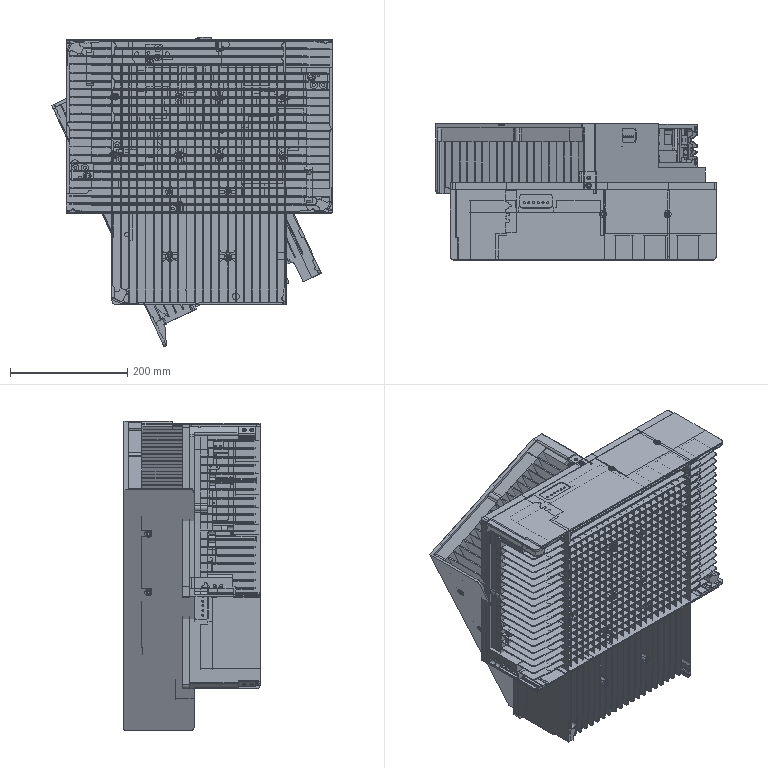CAM job | NX | 3-axis milling, drilling | stock box 478.438 x 232 x 527.231 mm
Tools:
number,name,description,diameter,corner_radius,flute_length,length,flutes
1,D10_J,Milling Tool-5 Parameters,10.0,0.0,50.0,50.0,2
2,CR_8,Countersink,8.0,0.0,0.0,60.0,2
3,CR_4,Countersink,4.0,0.0,0.0,60.0,2
4,D6_J,Milling Tool-5 Parameters,6.0,0.0,50.0,50.0,2
5,D4_J,Milling Tool-5 Parameters,4.0,0.0,50.0,60.0,2
6,Z2.6,Drilling Tool,2.6,0.0,30.0,50.0,2
7,M3,Drilling Tool,3.0,0.0,30.0,50.0,2
8,Z5.2,Drilling Tool,5.2,0.0,50.0,70.0,2
9,M6,Drilling Tool,6.0,0.0,30.0,50.0,2
17,M12X1.5,Drilling Tool,12.0,0.0,30.0,50.0,2
16,GSLT-M5,Drilling Tool,6.0,0.0,30.0,50.0,2
10,CR_3,Milling Tool-5 Parameters,0.3,0.0,50.0,75.0,2
11,Z10.5,Drilling Tool,10.5,0.0,50.0,70.0,2
12,D2.5_J,Milling Tool-5 Parameters,2.5,0.0,50.0,50.0,2
14,Z3.8,Drilling Tool,3.8,0.0,35.0,50.0,2
15,D3_J,Milling Tool-5 Parameters,3.0,0.0,30.0,50.0,2
16,D8R1,Milling Tool-5 Parameters,8.0,1.0,50.0,75.0,2
Operations:
program,operation,operation_type,tool,method,geometry_group,spindle_rpm,surface_speed,feed_per_tooth,feed_cut,feed_plunge,cut_length_mm,path_length_mm,cut_time_min,machine_time_min
W27,PLANAR_PROFILE_COPY_COPY_3_COPY_COPY,PlanarMilling,D10_J,METHOD,G54,7500.0,0.0,0.1,1500.0,100.0,47.6,102.4,0.0317,0.0372
W27,PLANAR_PROFILE_COPY_COPY_3_COPY,PlanarMilling,D10_J,METHOD,G54,7500.0,0.0,0.1,1500.0,100.0,186.0,896.277,0.124,0.195
W27,PX_1_COPY,SurfaceContour,D10_J,METHOD,G54,7500.0,69.0,0.2727,2500.0,100.0,630.219,773.27,0.2521,0.2664
W27,PLANAR_PROFILE_COPY,PlanarMilling,D10_J,METHOD,G54,7500.0,0.0,0.1667,2500.0,100.0,2403.044,2529.843,0.9612,0.9739
W27,PLANAR_PROFILE_COPY_COPY_2,PlanarMilling,D10_J,METHOD,G54,7500.0,0.0,0.1667,2500.0,100.0,854.585,981.385,0.3418,0.3545
W27,PLANAR_PROFILE_COPY_COPY_2_COPY_1,PlanarMilling,D10_J,METHOD,G54,7500.0,0.0,0.1,1500.0,100.0,521.673,638.673,0.3478,0.3595
W27,PLANAR_PROFILE_COPY_COPY_2_COPY_1_COPY,PlanarMilling,D10_J,METHOD,G54,7500.0,0.0,0.1,1500.0,100.0,35.267,305.732,0.0235,0.0506
W27,PLANAR_PROFILE_COPY_COPY_2_COPY,PlanarMilling,D10_J,METHOD,G54,7500.0,0.0,0.1667,2500.0,100.0,943.144,1069.944,0.3773,0.3899
W27,PLANAR_PROFILE_COPY_COPY_2_COPY_COPY,PlanarMilling,D10_J,METHOD,G54,7500.0,0.0,0.1667,2500.0,100.0,345.704,454.504,0.1383,0.1492
W27,PLANAR_PROFILE_COPY_COPY_3_COPY_2,PlanarMilling,D10_J,METHOD,G54,7500.0,0.0,0.1,1500.0,100.0,118.82,243.82,0.0792,0.0917
W27,PLANAR_PROFILE_COPY_COPY_3,PlanarMilling,D10_J,METHOD,G54,7500.0,0.0,0.1,1500.0,100.0,122.525,247.525,0.0817,0.0942
W27,PLANAR_MILL_COPY_COPY_COPY_1_COPY_COPY_COPY_1_COPY_COPY_COPY_COPY_1,PlanarMilling,D10_J,METHOD,G54,8000.0,0.0,0.2333,1500.0,100.0,736.062,861.062,0.4907,0.5032
W27,FACE_MILLING_COPY_COPY_COPY_1_COPY_3,FaceMilling,D10_J,METHOD,G54,8000.0,0.0,0.2333,1500.0,100.0,392.088,614.324,0.2614,0.2836
W27,FACE_MILLING_COPY_COPY_COPY_1_COPY_3_COPY,FaceMilling,D10_J,METHOD,G54,8000.0,0.0,0.2333,1500.0,100.0,317.508,966.305,0.2117,0.2766
W27,PX_1_COPY_COPY_1,SurfaceContour,D10_J,METHOD,G54,7500.0,69.0,0.2727,2500.0,100.0,485.34,561.34,0.1941,0.2017
W27,PLANAR_MILL_COPY_COPY_COPY_1_COPY_COPY_COPY_1_COPY_COPY_COPY_COPY_1_COPY,PlanarMilling,D10_J,METHOD,G54,8000.0,0.0,0.2333,1500.0,100.0,791.735,911.235,0.5278,0.5398
W27,PLANAR_PROFILE_COPY_COPY_COPY_COPY_COPY_COPY_COPY_1,PlanarMilling,D10_J,METHOD,G54,7500.0,0.0,0.08,1200.0,100.0,19.0,122.0,0.0158,0.0261
W27,DG_1_COPY_COPY_2_COPY,ZLevelMilling,D10_J,METHOD,G54,8500.0,0.0,0.1471,2500.0,100.0,935.965,1017.165,0.3744,0.3825
W27,FACE_MILLING_COPY_COPY_COPY_1_COPY_3_COPY_COPY,FaceMilling,D10_J,METHOD,G54,8000.0,0.0,0.2333,1500.0,100.0,196.507,801.996,0.131,0.1916
W27,DG_1_COPY_COPY_2_COPY_COPY_COPY_1,ZLevelMilling,D10_J,METHOD,G54,8500.0,0.0,0.1471,2500.0,100.0,955.229,1070.629,0.3821,0.3936
W27,DG_1_COPY_COPY_2_COPY_COPY,ZLevelMilling,D10_J,METHOD,G54,8500.0,0.0,0.1471,2500.0,100.0,1318.762,1434.162,0.5275,0.539
W27,HOLE_MILLING_3,CylinderMilling,D10_J,METHOD,G54,8000.0,0.0,0.0,2500.0,100.0,930.302,990.802,0.3721,0.3782
W27,HOLE_MILLING_3_COPY,CylinderMilling,D10_J,METHOD,G54,8000.0,0.0,0.0,1200.0,100.0,21.677,103.677,0.0181,0.0263
W27_COPY,HOLE_MILLING_3_COPY_1,CylinderMilling,D4_J,METHOD,G54,8000.0,0.0,0.0,2500.0,100.0,1240.867,1371.367,0.4963,0.5094
W27_COPY,HOLE_MILLING_3_COPY_1_COPY,CylinderMilling,D4_J,METHOD,G54,8000.0,0.0,0.0,2500.0,100.0,906.876,1037.376,0.3628,0.3758
W27_COPY,PLANAR_PROFILE_COPY_COPY_3_COPY_1,PlanarMilling,D4_J,METHOD,G54,7500.0,0.0,0.1,1500.0,100.0,511.204,656.514,0.3408,0.3553
W27_COPY,PLANAR_PROFILE_COPY_COPY_3_COPY_1_COPY,PlanarMilling,D4_J,METHOD,G54,7500.0,0.0,0.1,1500.0,100.0,176.817,227.742,0.1179,0.123
W65,ZK_1_COPY_COPY_4,Operation,CR_8,METHOD,G54,7500.0,0.0,0.0008,500.0,0.0,18.0,462.606,0.036,0.0805
W66,ZK_1_COPY_COPY_4_COPY,Operation,Z10.5,METHOD,G54,2000.0,0.0,0.0008,500.0,0.0,17.0,159.4,0.034,0.0482
W67,ZK_1_COPY_COPY_4_COPY_COPY,Operation,Z2.6,METHOD,G54,2000.0,0.0,0.0008,220.0,0.0,60.0,335.681,0.2727,0.3003
W68,DG_1_COPY_COPY_2_COPY_COPY_3,ZLevelMilling,D6_J,METHOD,G54,8500.0,0.0,0.0882,1500.0,100.0,967.287,1048.487,0.6449,0.653
W68,DG_1_COPY_COPY_2_COPY_COPY_COPY,ZLevelMilling,D6_J,METHOD,G54,8500.0,0.0,0.0882,1500.0,100.0,1853.936,1969.336,1.236,1.248
W68,DG_1_COPY_COPY_2_COPY_COPY_COPY_COPY,ZLevelMilling,D6_J,METHOD,G54,8500.0,0.0,0.1471,2500.0,100.0,663.86,1057.072,0.2655,0.3049
W68,DG_1_COPY_COPY_2_COPY_COPY_COPY_COPY_COPY,ZLevelMilling,D6_J,METHOD,G54,8500.0,0.0,0.1176,2000.0,100.0,1683.898,1802.898,0.8419,0.8538
W68,PLANAR_PROFILE_COPY_COPY_COPY_COPY_COPY_COPY,PlanarMilling,D6_J,METHOD,G54,7500.0,0.0,0.08,1200.0,100.0,118.212,275.212,0.0985,0.1142
W68,DG_1_COPY_COPY_2_COPY_COPY_COPY_COPY_COPY_COPY_COPY_COPY_COPY,ZLevelMilling,D6_J,METHOD,G54,8500.0,0.0,0.0882,1500.0,100.0,270.01,375.01,0.18,0.1905
W68,DG_1_COPY_COPY_2_COPY_COPY_COPY_COPY_COPY_COPY,ZLevelMilling,D6_J,METHOD,G54,8500.0,0.0,0.0882,1500.0,100.0,1167.785,1564.689,0.7785,0.8182
W68,DG_1_COPY_COPY_2_COPY_COPY_COPY_COPY_COPY_COPY_COPY,ZLevelMilling,D6_J,METHOD,G54,8500.0,0.0,0.0882,1500.0,100.0,434.204,683.626,0.2895,0.3144
W68,DG_1_COPY_COPY_2_COPY_COPY_COPY_COPY_COPY_COPY_COPY_COPY,ZLevelMilling,D6_J,METHOD,G54,8500.0,0.0,0.0882,1500.0,100.0,215.619,326.369,0.1437,0.1548
W68,PLANAR_PROFILE_COPY_COPY_COPY_COPY_COPY_COPY_COPY,PlanarMilling,D6_J,METHOD,G54,7500.0,0.0,0.1667,2500.0,100.0,355.477,496.477,0.1422,0.1563
W68,PLANAR_PROFILE_COPY_COPY_COPY_COPY_COPY_COPY_COPY_COPY,PlanarMilling,D6_J,METHOD,G54,7500.0,0.0,0.1667,2500.0,100.0,530.789,671.789,0.2123,0.2264
W68,PLANAR_MILL_COPY_COPY_COPY_1_COPY_COPY_COPY_1_COPY_COPY_COPY_COPY_1_COPY_1,PlanarMilling,D6_J,METHOD,G54,8000.0,0.0,0.2333,1500.0,100.0,525.616,934.317,0.3504,0.3913
W69,ZK_1_COPY_COPY_4_COPY_COPY_COPY,Operation,CR_8,METHOD,G54,7500.0,0.0,0.0008,500.0,0.0,17.5,250.681,0.035,0.0583
W71,ZK_1_COPY_COPY_4_COPY_COPY_COPY_1,Operation,M3,METHOD,G54,2000.0,0.0,0.0001,0.5,0.0,47.5,310.681,95.0,95.026
W72,DJ_COPY_COPY,PlanarMilling,CR_4,METHOD,G54,8500.0,0.0,0.1471,2500.0,100.0,130.576,348.576,0.0522,0.074
W72,DJ_COPY_COPY_COPY_1,PlanarMilling,CR_4,METHOD,G54,8500.0,0.0,0.1471,2500.0,100.0,82.266,136.266,0.0329,0.0383
W72,DJ_COPY_COPY_COPY,PlanarMilling,CR_4,METHOD,G54,8500.0,0.0,0.1471,2500.0,100.0,97.623,360.364,0.039,0.0653
W72,DJ_COPY_COPY_COPY_COPY,PlanarMilling,CR_4,METHOD,G54,8500.0,0.0,0.1471,2500.0,100.0,53.559,159.959,0.0214,0.0321
W72,DJ_COPY_COPY_COPY_COPY_COPY_COPY,PlanarMilling,CR_4,METHOD,G54,8500.0,0.0,0.1471,2500.0,100.0,18.398,120.798,0.0074,0.0176
W72,DJ_COPY_COPY_COPY_COPY_COPY,PlanarMilling,CR_4,METHOD,G54,8500.0,0.0,0.1471,2500.0,100.0,168.49,275.19,0.0674,0.0781
W74,DJ_COPY_COPY_COPY_2,PlanarMilling,CR_3,METHOD,G54,8500.0,0.0,0.0588,1000.0,100.0,316.906,2018.803,0.3169,0.4871
W74,DJ_COPY_COPY_COPY_2_COPY,PlanarMilling,CR_3,METHOD,G54,8500.0,0.0,0.0588,1000.0,100.0,72.086,843.529,0.0721,0.1492
W74,DJ_COPY_COPY_COPY_2_COPY_2,PlanarMilling,CR_3,METHOD,G54,8500.0,0.0,0.0588,1000.0,100.0,14.005,128.805,0.014,0.0255
W73,ZK_1_COPY_COPY_4_COPY_COPY_1,Operation,M12X1.5,METHOD,G54,2000.0,0.0,0.0004,1.5,0.0,12.0,149.4,8.0,8.014
W73_COPY,PLANAR_PROFILE_COPY_COPY_3_COPY_1_COPY_COPY,PlanarMilling,D4_J,METHOD,G54,7500.0,0.0,0.1,1500.0,100.0,176.817,227.742,0.1179,0.123
W73_COPY,DJ_COPY_COPY_COPY_2_COPY_2_COPY,PlanarMilling,CR_3,METHOD,G54,8500.0,0.0,0.0588,1000.0,100.0,14.005,128.805,0.014,0.0255
W73_COPY,DG_1_COPY_COPY_2_COPY_COPY_COPY_COPY_COPY_1,ZLevelMilling,D8R1,METHOD,G54,8000.0,251.0,0.125,2000.0,100.0,469.925,596.616,0.235,0.2476
W02,FACE_MILLING_COPY_COPY_COPY_1_COPY_3_COPY_1,FaceMilling,D10_J,METHOD,G54,8000.0,0.0,0.2333,1500.0,100.0,116.203,294.447,0.0775,0.0953
W02,PLANAR_PROFILE_COPY_COPY_3_COPY_COPY_COPY,PlanarMilling,D10_J,METHOD,G54,8000.0,0.0,0.1562,2500.0,100.0,302.884,502.873,0.1212,0.1412
W02,PLANAR_MILL_COPY_COPY_COPY_1_COPY_COPY_COPY_1_COPY_COPY_COPY_COPY_1_COPY_2,PlanarMilling,D10_J,METHOD,G54,8000.0,0.0,0.2333,1500.0,100.0,652.682,814.615,0.4351,0.4513
W03,HOLE_MILLING,CylinderMilling,D4_J,METHOD,G54,8000.0,100.0,0.0938,1500.0,100.0,194.81,385.41,0.1299,0.1489
W04,ZK_1_COPY_COPY_4_COPY_1,Operation,CR_8,METHOD,G54,7500.0,0.0,0.0008,500.0,0.0,6.0,166.618,0.012,0.0281
W05,ZK_1_COPY_COPY_4_COPY_1_COPY,Operation,Z5.2,METHOD,G54,3000.0,0.0,0.0008,300.0,0.0,32.0,218.618,0.1067,0.1253
W06,ZK_1_COPY_COPY_4_COPY_1_COPY_1,Operation,CR_8,METHOD,G54,7500.0,0.0,0.0008,500.0,0.0,10.0,174.618,0.02,0.0365
W12,ZK_1_COPY_COPY_4_COPY_1_COPY_COPY,Operation,M6,METHOD,G54,2000.0,0.0,0.0008,1.0,0.0,26.0,206.618,26.0,26.018
W13,DJ_COPY_COPY_COPY_3,PlanarMilling,CR_4,METHOD,G54,8500.0,0.0,0.1471,2500.0,100.0,140.407,407.063,0.0562,0.0828
W01,PLANAR_MILL_COPY_COPY_COPY_1_COPY_COPY_COPY_1_COPY_COPY_COPY_COPY_1_COPY_COPY,PlanarMilling,D10_J,METHOD,G54,8000.0,0.0,0.2333,1500.0,100.0,1618.01,1674.01,1.079,1.084
W01,PLANAR_MILL_COPY_COPY_COPY_1_COPY_COPY_COPY_1_COPY_COPY_COPY_COPY_1_COPY_COPY_COPY,PlanarMilling,D10_J,METHOD,G54,8000.0,0.0,0.2333,1500.0,100.0,1170.544,1221.544,0.7804,0.7855
W01,PLANAR_MILL_COPY_COPY_COPY_1_COPY_COPY_COPY_1_COPY_COPY_COPY_COPY_1_COPY_COPY_COPY_COPY,PlanarMilling,D10_J,METHOD,G54,8000.0,0.0,0.2333,1500.0,100.0,1163.605,1226.105,0.7757,0.782
W01,FACE_MILLING_COPY_COPY_COPY_1_COPY_3_COPY_2,FaceMilling,D10_J,METHOD,G54,8000.0,0.0,0.2333,1500.0,100.0,1782.698,2104.083,1.188,1.221
W01,CAVITY_MILL,CavityMilling,D10_J,METHOD,G54,7500.0,235.0,0.2333,3500.0,100.0,47087.83,49581.844,13.454,13.703
W01,FACE_MILLING_COPY_COPY_COPY_1_COPY_3_COPY_2_COPY,FaceMilling,D10_J,METHOD,G54,8000.0,0.0,0.2333,1500.0,100.0,1344.186,2793.189,0.8961,1.041
W07,HOLE_MILLING_1,CylinderMilling,D6_J,METHOD,G54,8000.0,0.0,0.0,1500.0,100.0,216.836,303.836,0.1446,0.1533
W07,CAVITY_MILL_COPY,CavityMilling,D6_J,METHOD,G54,8000.0,150.0,0.1875,3000.0,100.0,16037.881,26925.285,5.346,6.435
W07,FACE_MILLING_COPY_COPY_COPY_1_COPY_3_COPY_2_COPY_COPY,FaceMilling,D6_J,METHOD,G54,8000.0,0.0,0.2333,1500.0,100.0,858.792,2126.935,0.5725,0.6993
W07,PLANAR_PROFILE_COPY_COPY_3_COPY_COPY_1_COPY_3,PlanarMilling,D6_J,METHOD,G54,7500.0,0.0,0.1,1500.0,100.0,88.083,162.083,0.0587,0.0661
W07,FACE_MILLING_COPY_COPY_COPY_1_COPY_3_COPY_2_COPY_COPY_COPY,FaceMilling,D6_J,METHOD,G54,8000.0,0.0,0.2333,1500.0,100.0,608.245,1917.272,0.4055,0.5364
W07,PLANAR_PROFILE_COPY_COPY_3_COPY_COPY_1,PlanarMilling,D6_J,METHOD,G54,7500.0,0.0,0.1,1500.0,100.0,568.85,773.65,0.3792,0.3997
W07,PLANAR_PROFILE_COPY_COPY_3_COPY_COPY_1_COPY,PlanarMilling,D6_J,METHOD,G54,7500.0,0.0,0.1,1500.0,100.0,21.283,137.683,0.0142,0.0258
W07,PLANAR_PROFILE_COPY_COPY_3_COPY_COPY_1_COPY_1,PlanarMilling,D6_J,METHOD,G54,7500.0,0.0,0.1,1500.0,100.0,402.733,998.933,0.2685,0.3281
W07,FACE_MILLING_COPY_COPY_COPY_1_COPY_3_COPY_2_COPY_COPY_COPY_3,FaceMilling,D6_J,METHOD,G54,8000.0,0.0,0.2188,3500.0,100.0,1632.647,1869.109,0.4665,0.4901
W07,FACE_MILLING_COPY_COPY_COPY_1_COPY_3_COPY_2_COPY_COPY_COPY_3_COPY,FaceMilling,D6_J,METHOD,G54,8000.0,0.0,0.2333,1500.0,100.0,356.654,394.454,0.2378,0.2415
W07,DG_1_COPY_COPY_2_COPY_COPY_1,ZLevelMilling,D6_J,METHOD,G54,8500.0,0.0,0.1471,2500.0,100.0,2918.479,5757.108,1.167,1.451
W07,PX_1_COPY_COPY,SurfaceContour,D6_J,METHOD,G54,7500.0,69.0,0.2727,2500.0,100.0,3224.559,3765.461,1.29,1.344
W08,FACE_MILLING_COPY_COPY_COPY_1_COPY_3_COPY_2_COPY_COPY_COPY_2_COPY_COPY,FaceMilling,D4_J,METHOD,G54,8000.0,0.0,0.2333,1500.0,100.0,125.867,468.46,0.0839,0.1182
W08,DG_1_COPY_COPY_2_COPY_COPY_1_COPY,ZLevelMilling,D4_J,METHOD,G54,8500.0,0.0,0.1471,2500.0,100.0,6784.364,7077.339,2.714,2.743
W08,DG_1_COPY_COPY_2_COPY_COPY_1_COPY_COPY,ZLevelMilling,D4_J,METHOD,G54,8500.0,0.0,0.1471,2500.0,100.0,1548.077,1712.238,0.6192,0.6356
W08,PLANAR_PROFILE_COPY_COPY_3_COPY_COPY_1_COPY_2,PlanarMilling,D4_J,METHOD,G54,7500.0,0.0,0.1,1500.0,100.0,522.0,627.444,0.348,0.3585
W08,PLANAR_PROFILE_COPY_COPY_3_COPY_COPY_1_COPY_2_COPY,PlanarMilling,D4_J,METHOD,G54,7500.0,0.0,0.1667,2500.0,100.0,2057.213,2378.148,0.8229,0.855
W08,FACE_MILLING_COPY_COPY_COPY_1_COPY_3_COPY_2_COPY_COPY_COPY_1,FaceMilling,D4_J,METHOD,G54,8000.0,0.0,0.2333,1500.0,100.0,99.01,362.088,0.066,0.0923
W08,PLANAR_PROFILE_COPY_COPY_3_COPY_COPY_1_COPY_2_COPY_COPY,PlanarMilling,D4_J,METHOD,G54,7500.0,0.0,0.1,1500.0,100.0,43.783,133.783,0.0292,0.0382
W08,PLANAR_PROFILE_COPY_COPY_3_COPY_COPY_1_COPY_3_COPY,PlanarMilling,D4_J,METHOD,G54,7500.0,0.0,0.1,1500.0,100.0,95.954,169.954,0.064,0.0714
W08,PX_1_COPY_COPY_COPY,SurfaceContour,D4_J,METHOD,G54,7500.0,69.0,0.2727,2500.0,100.0,996.115,1109.056,0.3984,0.4097
W08,PX_1_COPY_COPY_COPY_COPY,SurfaceContour,D4_J,METHOD,G54,7500.0,69.0,0.1,1500.0,100.0,92.736,199.936,0.0618,0.0725
W08,PLANAR_PROFILE_COPY_COPY_3_COPY_COPY_1_COPY_3_COPY_1,PlanarMilling,D4_J,METHOD,G54,7500.0,0.0,0.1,1500.0,100.0,28.283,72.283,0.0189,0.0233
W14,PLANAR_MILL_COPY_COPY_COPY_1_COPY_COPY_COPY_1_COPY_COPY_COPY_COPY_1_COPY_COPY_COPY_COPY_COPY_COPY_COPY_1_COPY_COPY,PlanarMilling,D2.5_J,METHOD,G54,8000.0,0.0,0.0938,1500.0,100.0,115.791,219.312,0.0772,0.0875
W14,PLANAR_MILL_COPY_COPY_COPY_1_COPY_COPY_COPY_1_COPY_COPY_COPY_COPY_1_COPY_COPY_COPY_COPY_COPY,PlanarMilling,D2.5_J,METHOD,G54,8000.0,0.0,0.1562,2500.0,100.0,5609.504,5689.004,2.244,2.252
W14,PLANAR_MILL_COPY_COPY_COPY_1_COPY_COPY_COPY_1_COPY_COPY_COPY_COPY_1_COPY_COPY_COPY_COPY_COPY_COPY,PlanarMilling,D2.5_J,METHOD,G54,8000.0,0.0,0.1562,2500.0,100.0,301.593,405.305,0.1206,0.131
W14,PLANAR_MILL_COPY_COPY_COPY_1_COPY_COPY_COPY_1_COPY_COPY_COPY_COPY_1_COPY_COPY_COPY_COPY_COPY_COPY_COPY,PlanarMilling,D2.5_J,METHOD,G54,8000.0,0.0,0.1562,2500.0,100.0,301.593,405.305,0.1206,0.131
W14,PLANAR_MILL_COPY_COPY_COPY_1_COPY_COPY_COPY_1_COPY_COPY_COPY_COPY_1_COPY_COPY_COPY_COPY_COPY_COPY_COPY_1,PlanarMilling,D2.5_J,METHOD,G54,8000.0,0.0,0.1562,2500.0,100.0,301.593,405.305,0.1206,0.131
W14,PLANAR_MILL_COPY_COPY_COPY_1_COPY_COPY_COPY_1_COPY_COPY_COPY_COPY_1_COPY_COPY_COPY_COPY_COPY_COPY_COPY_1_COPY,PlanarMilling,D2.5_J,METHOD,G54,8000.0,0.0,0.1562,2500.0,100.0,301.593,405.305,0.1206,0.131
W15,ZK_1_COPY_COPY_4_COPY_2,Operation,CR_8,METHOD,G54,7500.0,0.0,0.0008,500.0,0.0,42.0,602.9,0.084,0.1401
W16,ZK_1_COPY_COPY_4_COPY_COPY_COPY_2,Operation,Z2.6,METHOD,G54,2000.0,0.0,0.0008,220.0,0.0,24.0,190.859,0.1091,0.1258
W16,ZK_1_COPY_COPY_4_COPY_COPY_COPY_2_COPY,Operation,Z2.6,METHOD,G54,2000.0,0.0,0.0008,220.0,0.0,42.0,218.404,0.1909,0.2085
W25,ZK_1_COPY_COPY_4_COPY_COPY_COPY_2_COPY_COPY,Operation,Z3.8,METHOD,G54,2000.0,0.0,0.0008,220.0,0.0,30.0,192.034,0.1364,0.1526
W25,ZK_1_COPY_COPY_4_COPY_COPY_COPY_2_COPY_COPY_1,Operation,Z3.8,METHOD,G54,2000.0,0.0,0.0008,220.0,0.0,72.0,254.668,0.3273,0.3455
W26,HOLE_MILLING_2,CylinderMilling,D3_J,METHOD,G54,8000.0,0.0,0.0,1500.0,100.0,732.813,960.313,0.4885,0.5113
W26,DG_1_COPY_COPY_2_COPY_COPY_1_COPY_COPY_1,ZLevelMilling,D3_J,METHOD,G54,8500.0,0.0,0.1176,2000.0,100.0,538.012,737.175,0.269,0.2889
W28,ZK_1_COPY_COPY_4_COPY_COPY_COPY_2_COPY_COPY_2,Operation,CR_8,METHOD,G54,2000.0,0.0,0.0008,220.0,0.0,21.0,296.974,0.0955,0.1231
W28,ZK_1_COPY_COPY_4_COPY_COPY_COPY_2_COPY_COPY_COPY,Operation,CR_8,METHOD,G54,2000.0,0.0,0.0008,220.0,0.0,9.0,150.034,0.0409,0.055
W28,ZK_1_COPY_COPY_4_COPY_COPY_COPY_2_COPY_COPY_1_COPY,Operation,CR_8,METHOD,G54,2000.0,0.0,0.0008,220.0,0.0,23.4,157.468,0.1064,0.1198
W29,DJ_COPY_COPY_COPY_4,PlanarMilling,CR_4,METHOD,G54,8500.0,0.0,0.1471,2500.0,100.0,415.091,607.277,0.166,0.1853
W29,DJ_COPY_COPY_COPY_4_COPY,PlanarMilling,CR_4,METHOD,G54,8500.0,0.0,0.1471,2500.0,100.0,125.111,193.511,0.05,0.0569
W29,DJ_COPY_COPY_COPY_4_COPY_COPY,PlanarMilling,CR_4,METHOD,G54,8500.0,0.0,0.1471,2500.0,100.0,400.018,468.418,0.16,0.1668
W29,DJ_COPY_COPY_COPY_4_COPY_COPY_COPY,PlanarMilling,CR_4,METHOD,G54,8500.0,0.0,0.1471,2500.0,100.0,113.1,211.3,0.0452,0.0551
W29,DJ_COPY_COPY_COPY_4_COPY_COPY_COPY_COPY,PlanarMilling,CR_4,METHOD,G54,8500.0,0.0,0.1471,2500.0,100.0,65.996,146.797,0.0264,0.0345
W29,DJ_COPY_COPY_COPY_4_COPY_COPY_COPY_COPY_COPY,PlanarMilling,CR_4,METHOD,G54,8500.0,0.0,0.1471,2500.0,100.0,53.741,140.741,0.0215,0.0302
W29,DJ_COPY_COPY_COPY_4_COPY_COPY_COPY_COPY_COPY_COPY,PlanarMilling,CR_4,METHOD,G54,8500.0,0.0,0.1471,2500.0,100.0,113.785,358.999,0.0455,0.07
W30,DJ_COPY_COPY_COPY_2_COPY_1,PlanarMilling,CR_3,METHOD,G54,8500.0,0.0,0.0588,1000.0,100.0,110.225,766.258,0.1102,0.1758
W30,DJ_COPY_COPY_COPY_2_COPY_1_COPY,PlanarMilling,CR_3,METHOD,G54,8500.0,0.0,0.0588,1000.0,100.0,39.77,374.539,0.0398,0.0732
W30,DJ_COPY_COPY_COPY_2_COPY_1_COPY_2,PlanarMilling,CR_3,METHOD,G54,8500.0,0.0,0.0588,1000.0,100.0,58.322,322.625,0.0583,0.0848
W30,DJ_COPY_COPY_COPY_2_COPY_1_COPY_COPY,PlanarMilling,CR_3,METHOD,G54,8500.0,0.0,0.0588,1000.0,100.0,17.192,196.224,0.0172,0.0351
W31,ZK_1_COPY_COPY_4_COPY_COPY_COPY_2_COPY_COPY_COPY_1,Operation,GSLT-M5,METHOD,G54,1000.0,0.0,0.0008,0.8,0.0,29.6,191.234,37.0,37.016
W32,ZK_1_COPY_COPY_4_COPY_COPY_COPY_2_COPY_1_COPY,Operation,M3,METHOD,G54,2000.0,0.0,0.0001,0.5,0.0,20.0,182.859,40.0,40.016
W32,ZK_1_COPY_COPY_4_COPY_COPY_COPY_2_COPY_COPY_3_COPY,Operation,M3,METHOD,G54,2000.0,0.0,0.0001,0.5,0.0,34.0,202.404,68.0,68.017
W09,ZK_1_COPY_COPY_4_COPY_1_COPY_2,Operation,CR_8,METHOD,G54,7500.0,0.0,0.0008,500.0,0.0,6.0,67.153,0.012,0.0181
W10,ZK_1_COPY_COPY_4_COPY_1_COPY_COPY_1,Operation,Z5.2,METHOD,G54,3000.0,0.0,0.0008,300.0,0.0,42.0,139.153,0.14,0.1497
W11,ZK_1_COPY_COPY_4_COPY_1_COPY_1_COPY,Operation,CR_8,METHOD,G54,7500.0,0.0,0.0008,500.0,0.0,10.0,75.153,0.02,0.0265
W18,ZK_1_COPY_COPY_4_COPY_1_COPY_COPY_COPY,Operation,M6,METHOD,G54,2000.0,0.0,0.0008,1.0,0.0,32.0,119.153,32.0,32.009
NC_PROGRAM,HOLE_MILLING_4,CylinderMilling,D4_J,METHOD,G54,2500.0,0.0,0.0,1000.0,100.0,1907.007,1961.907,1.907,1.913
Q01,FACE_MILLING_COPY_COPY_COPY_1_COPY_3_COPY_COPY_1,FaceMilling,D6_J,METHOD,G54,8000.0,0.0,0.2333,1500.0,100.0,748.02,1444.507,0.4987,0.5683
Q01,PLANAR_PROFILE_COPY_COPY_COPY_COPY_COPY_COPY_COPY_COPY_COPY,PlanarMilling,D6_J,METHOD,G54,8000.0,0.0,0.2333,1500.0,100.0,33.991,140.991,0.0227,0.0334